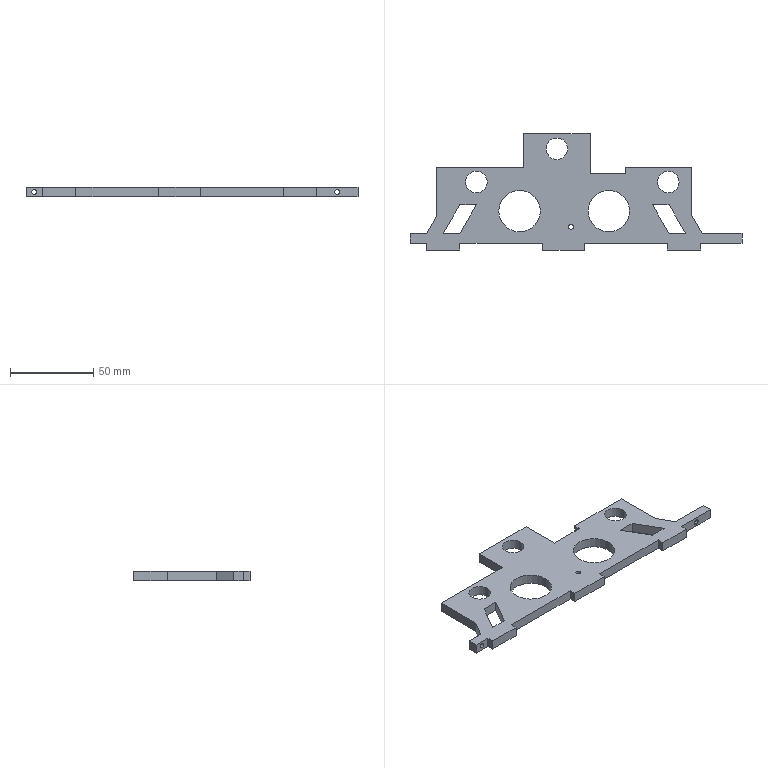Part | SolidWorks | features ICE 11, Extrusion 1 | 1 solid | 54 faces | box 200 x 70 x 6 mm | volume 39858 mm3 | plane 38 | cylinder 16 | commonest cylinder face diameters 3 x6 13 x6 25 x4